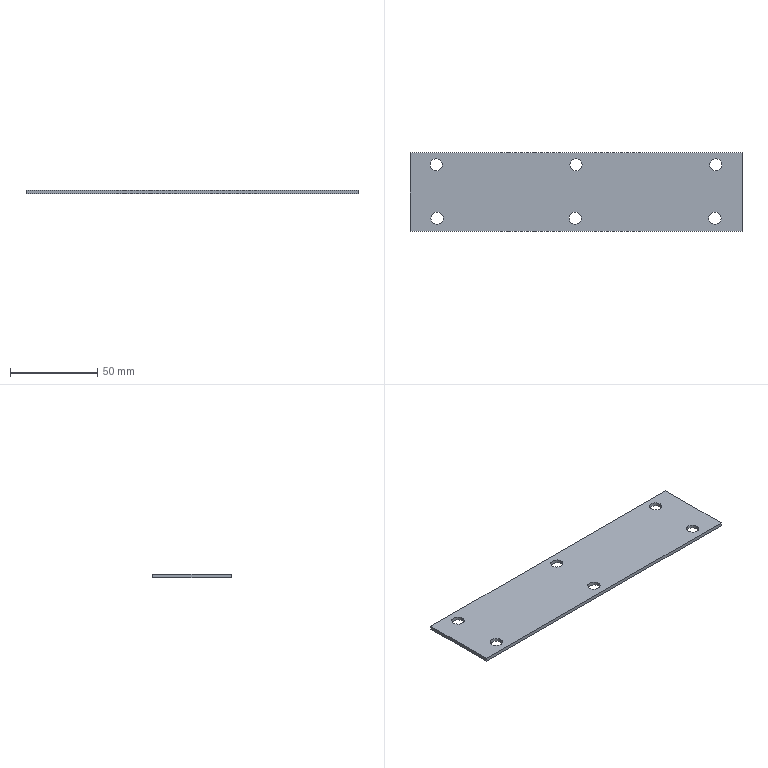Part | STEP file | 1_id1306_x_t | 1 solid | 18 faces | box 190 x 45 x 2 mm | volume 16638 mm3 | cylinder 12 | plane 6 | commonest cylinder face diameters 7 x12